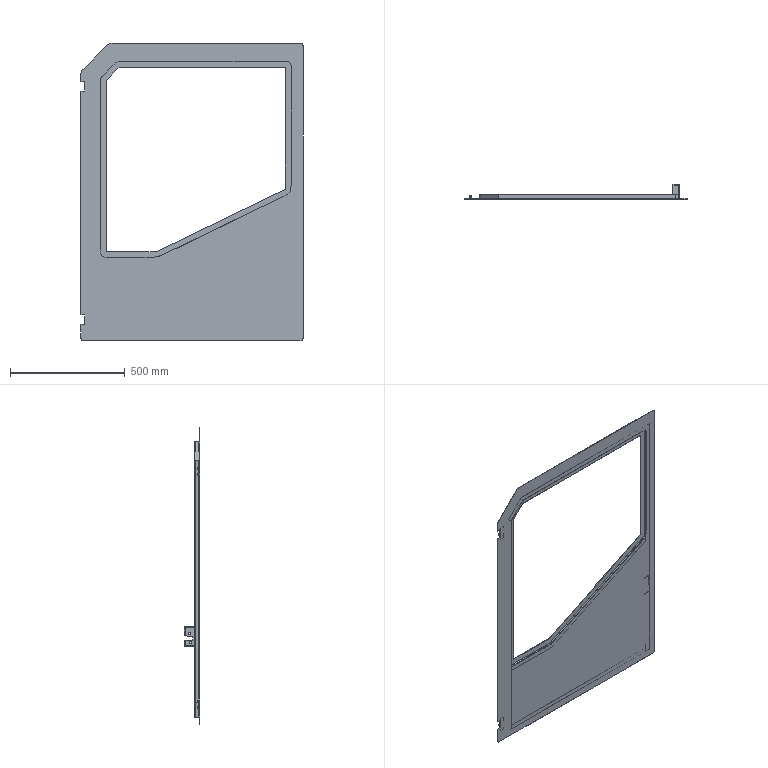Part | NX | features BREP 14 | 19 solids | 362 faces | volume 2123684 mm3 | plane 214 | cylinder 80 | cone 37 | spline 16 | torus 8 | sphere 7 | commonest cylinder face diameters 10 x18 5 x11 7.4 x8 8 x8 10.4 x8 6 x4